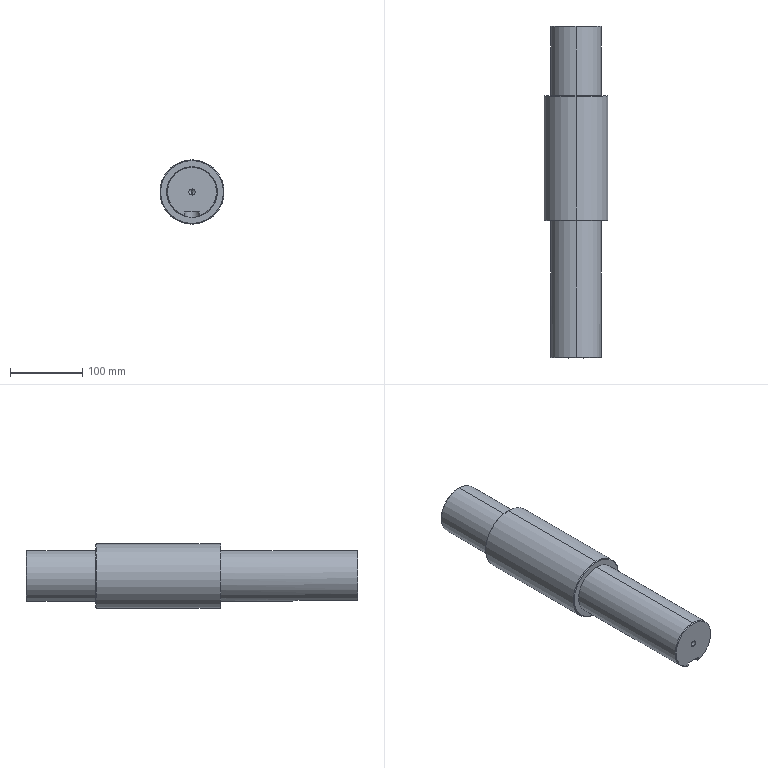Part | SolidWorks | features ICE 3, HoleWzd 2, Chamfer 1, Extrusion 1, MoveFace 1 | 1 solid | 30 faces | box 89 x 459.5 x 89 mm | volume 2162162 mm3 | cone 12 | cylinder 11 | plane 7 | commonest cylinder face diameters 8.5 x4 70 x4 89 x2 20 x1
STEP:
#1=CARTESIAN_POINT('',(0.,405.,-4.25));
#2=VERTEX_POINT('',#1);
#3=CARTESIAN_POINT('',(0.,405.,4.25));
#4=VERTEX_POINT('',#3);
#5=CARTESIAN_POINT('',(0.,405.,0.));
#6=DIRECTION('',(0.,1.,0.));
#7=DIRECTION('',(0.,0.,1.));
#8=AXIS2_PLACEMENT_3D('',#5,#6,#7);
#9=CIRCLE('',#8,4.25);
#10=EDGE_CURVE('',#2,#4,#9,.T.);
#11=ORIENTED_EDGE('',*,*,#10,.F.);
#12=CARTESIAN_POINT('',(0.,425.,-4.25));
#13=VERTEX_POINT('',#12);
#14=CARTESIAN_POINT('',(0.,425.,-4.25));
#15=DIRECTION('',(0.,1.,0.));
#16=VECTOR('',#15,1000.);
#17=LINE('',#14,#16);
#18=EDGE_CURVE('',#2,#13,#17,.T.);
#19=ORIENTED_EDGE('',*,*,#18,.T.);
#20=CARTESIAN_POINT('',(0.,425.,4.25));
#21=VERTEX_POINT('',#20);
#22=CARTESIAN_POINT('',(0.,425.,0.));
#23=DIRECTION('',(0.,1.,0.));
#24=DIRECTION('',(0.,0.,1.));
#25=AXIS2_PLACEMENT_3D('',#22,#23,#24);
#26=CIRCLE('',#25,4.25);
#27=EDGE_CURVE('',#13,#21,#26,.T.);
#28=ORIENTED_EDGE('',*,*,#27,.T.);
#29=CARTESIAN_POINT('',(0.,425.,4.25));
#30=DIRECTION('',(0.,1.,0.));
#31=VECTOR('',#30,1000.);
#32=LINE('',#29,#31);
#33=EDGE_CURVE('',#4,#21,#32,.T.);
#34=ORIENTED_EDGE('',*,*,#33,.F.);
#35=EDGE_LOOP('',(#11,#19,#28,#34));
#36=FACE_OUTER_BOUND('',#35,.T.);
#37=CARTESIAN_POINT('',(0.,425.,0.));
#38=DIRECTION('',(0.,1.,0.));
#39=DIRECTION('',(0.,0.,1.));
#40=AXIS2_PLACEMENT_3D('',#37,#38,#39);
#41=CYLINDRICAL_SURFACE('',#40,4.25);
#42=ADVANCED_FACE('',(#36),#41,.F.);
#43=CARTESIAN_POINT('',(0.,402.446,0.));
#44=VERTEX_POINT('',#43);
#45=CARTESIAN_POINT('',(0.,405.,4.25));
#46=DIRECTION('',(0.,0.515,0.8572));
#47=VECTOR('',#46,1000.);
#48=LINE('',#45,#47);
#49=EDGE_CURVE('',#44,#4,#48,.T.);
#50=ORIENTED_EDGE('',*,*,#49,.F.);
#51=CARTESIAN_POINT('',(0.,405.,-4.25));
#52=DIRECTION('',(0.,0.515,-0.8572));
#53=VECTOR('',#52,1000.);
#54=LINE('',#51,#53);
#55=EDGE_CURVE('',#44,#2,#54,.T.);
#56=ORIENTED_EDGE('',*,*,#55,.T.);
#57=ORIENTED_EDGE('',*,*,#10,.T.);
#58=EDGE_LOOP('',(#50,#56,#57));
#59=FACE_OUTER_BOUND('',#58,.T.);
#60=CARTESIAN_POINT('',(0.,405.,0.));
#61=DIRECTION('',(0.,1.,0.));
#62=DIRECTION('',(0.,0.,1.));
#63=AXIS2_PLACEMENT_3D('',#60,#61,#62);
#64=CONICAL_SURFACE('',#63,4.25,1.03);
#65=ADVANCED_FACE('',(#59),#64,.F.);
#66=CARTESIAN_POINT('',(0.,425.,34.));
#67=VERTEX_POINT('',#66);
#68=CARTESIAN_POINT('',(0.,425.,-34.));
#69=VERTEX_POINT('',#68);
#70=CARTESIAN_POINT('',(0.,425.,0.));
#71=DIRECTION('',(0.,1.,0.));
#72=DIRECTION('',(0.,0.,1.));
#73=AXIS2_PLACEMENT_3D('',#70,#71,#72);
#74=CIRCLE('',#73,34.);
#75=EDGE_CURVE('',#67,#69,#74,.T.);
#76=ORIENTED_EDGE('',*,*,#75,.F.);
#77=CARTESIAN_POINT('',(0.,424.,35.));
#78=VERTEX_POINT('',#77);
#79=CARTESIAN_POINT('',(0.,425.,34.));
#80=DIRECTION('',(0.,-0.7071,0.7071));
#81=VECTOR('',#80,1000.);
#82=LINE('',#79,#81);
#83=EDGE_CURVE('',#67,#78,#82,.T.);
#84=ORIENTED_EDGE('',*,*,#83,.T.);
#85=CARTESIAN_POINT('',(0.,424.,-35.));
#86=VERTEX_POINT('',#85);
#87=CARTESIAN_POINT('',(0.,424.,0.));
#88=DIRECTION('',(0.,-1.,0.));
#89=DIRECTION('',(0.,0.,1.));
#90=AXIS2_PLACEMENT_3D('',#87,#88,#89);
#91=CIRCLE('',#90,35.);
#92=EDGE_CURVE('',#86,#78,#91,.T.);
#93=ORIENTED_EDGE('',*,*,#92,.F.);
#94=CARTESIAN_POINT('',(0.,425.,-34.));
#95=DIRECTION('',(0.,-0.7071,-0.7071));
#96=VECTOR('',#95,1000.);
#97=LINE('',#94,#96);
#98=EDGE_CURVE('',#69,#86,#97,.T.);
#99=ORIENTED_EDGE('',*,*,#98,.F.);
#100=EDGE_LOOP('',(#76,#84,#93,#99));
#101=FACE_OUTER_BOUND('',#100,.T.);
#102=CARTESIAN_POINT('',(0.,425.,0.));
#103=DIRECTION('',(0.,-1.,0.));
#104=DIRECTION('',(0.,0.,-1.));
#105=AXIS2_PLACEMENT_3D('',#102,#103,#104);
#106=CONICAL_SURFACE('',#105,34.,0.7854);
#107=ADVANCED_FACE('',(#101),#106,.T.);
#108=CARTESIAN_POINT('',(0.,328.7,43.5));
#109=VERTEX_POINT('',#108);
#110=CARTESIAN_POINT('',(0.,328.7,-43.5));
#111=VERTEX_POINT('',#110);
#112=CARTESIAN_POINT('',(0.,328.7,0.));
#113=DIRECTION('',(0.,1.,0.));
#114=DIRECTION('',(0.,0.,1.));
#115=AXIS2_PLACEMENT_3D('',#112,#113,#114);
#116=CIRCLE('',#115,43.5);
#117=EDGE_CURVE('',#109,#111,#116,.T.);
#118=ORIENTED_EDGE('',*,*,#117,.F.);
#119=CARTESIAN_POINT('',(0.,327.7,44.5));
#120=VERTEX_POINT('',#119);
#121=CARTESIAN_POINT('',(0.,328.7,43.5));
#122=DIRECTION('',(0.,-0.7071,0.7071));
#123=VECTOR('',#122,1000.);
#124=LINE('',#121,#123);
#125=EDGE_CURVE('',#109,#120,#124,.T.);
#126=ORIENTED_EDGE('',*,*,#125,.T.);
#127=CARTESIAN_POINT('',(0.,327.7,-44.5));
#128=VERTEX_POINT('',#127);
#129=CARTESIAN_POINT('',(0.,327.7,0.));
#130=DIRECTION('',(0.,-1.,0.));
#131=DIRECTION('',(0.,0.,1.));
#132=AXIS2_PLACEMENT_3D('',#129,#130,#131);
#133=CIRCLE('',#132,44.5);
#134=EDGE_CURVE('',#128,#120,#133,.T.);
#135=ORIENTED_EDGE('',*,*,#134,.F.);
#136=CARTESIAN_POINT('',(0.,328.7,-43.5));
#137=DIRECTION('',(0.,-0.7071,-0.7071));
#138=VECTOR('',#137,1000.);
#139=LINE('',#136,#138);
#140=EDGE_CURVE('',#111,#128,#139,.T.);
#141=ORIENTED_EDGE('',*,*,#140,.F.);
#142=EDGE_LOOP('',(#118,#126,#135,#141));
#143=FACE_OUTER_BOUND('',#142,.T.);
#144=CARTESIAN_POINT('',(0.,328.7,0.));
#145=DIRECTION('',(0.,-1.,0.));
#146=DIRECTION('',(0.,0.,-1.));
#147=AXIS2_PLACEMENT_3D('',#144,#145,#146);
#148=CONICAL_SURFACE('',#147,43.5,0.7854);
#149=ADVANCED_FACE('',(#143),#148,.T.);
#150=CARTESIAN_POINT('',(0.,155.3,-43.5));
#151=VERTEX_POINT('',#150);
#152=CARTESIAN_POINT('',(0.,155.3,43.5));
#153=VERTEX_POINT('',#152);
#154=CARTESIAN_POINT('',(0.,155.3,0.));
#155=DIRECTION('',(0.,-1.,0.));
#156=DIRECTION('',(0.,0.,-1.));
#157=AXIS2_PLACEMENT_3D('',#154,#155,#156);
#158=CIRCLE('',#157,43.5);
#159=EDGE_CURVE('',#151,#153,#158,.T.);
#160=ORIENTED_EDGE('',*,*,#159,.F.);
#161=CARTESIAN_POINT('',(0.,156.3,-44.5));
#162=VERTEX_POINT('',#161);
#163=CARTESIAN_POINT('',(0.,155.3,-43.5));
#164=DIRECTION('',(0.,0.7071,-0.7071));
#165=VECTOR('',#164,1000.);
#166=LINE('',#163,#165);
#167=EDGE_CURVE('',#151,#162,#166,.T.);
#168=ORIENTED_EDGE('',*,*,#167,.T.);
#169=CARTESIAN_POINT('',(0.,156.3,44.5));
#170=VERTEX_POINT('',#169);
#171=CARTESIAN_POINT('',(0.,156.3,0.));
#172=DIRECTION('',(0.,1.,0.));
#173=DIRECTION('',(0.,0.,-1.));
#174=AXIS2_PLACEMENT_3D('',#171,#172,#173);
#175=CIRCLE('',#174,44.5);
#176=EDGE_CURVE('',#170,#162,#175,.T.);
#177=ORIENTED_EDGE('',*,*,#176,.F.);
#178=CARTESIAN_POINT('',(0.,155.3,43.5));
#179=DIRECTION('',(0.,0.7071,0.7071));
#180=VECTOR('',#179,1000.);
#181=LINE('',#178,#180);
#182=EDGE_CURVE('',#153,#170,#181,.T.);
#183=ORIENTED_EDGE('',*,*,#182,.F.);
#184=EDGE_LOOP('',(#160,#168,#177,#183));
#185=FACE_OUTER_BOUND('',#184,.T.);
#186=CARTESIAN_POINT('',(0.,155.3,0.));
#187=DIRECTION('',(0.,1.,0.));
#188=DIRECTION('',(0.,0.,1.));
#189=AXIS2_PLACEMENT_3D('',#186,#187,#188);
#190=CONICAL_SURFACE('',#189,43.5,0.7854);
#191=ADVANCED_FACE('',(#185),#190,.T.);
#192=CARTESIAN_POINT('',(0.,-34.5,34.));
#193=VERTEX_POINT('',#192);
#194=CARTESIAN_POINT('',(-10.,-34.5,-32.496));
#195=VERTEX_POINT('',#194);
#196=CARTESIAN_POINT('',(0.,-34.5,0.));
#197=DIRECTION('',(0.,-1.,0.));
#198=DIRECTION('',(0.,0.,1.));
#199=AXIS2_PLACEMENT_3D('',#196,#197,#198);
#200=CIRCLE('',#199,34.);
#201=EDGE_CURVE('',#193,#195,#200,.T.);
#202=ORIENTED_EDGE('',*,*,#201,.F.);
#203=CARTESIAN_POINT('',(0.,-33.5,35.));
#204=VERTEX_POINT('',#203);
#205=CARTESIAN_POINT('',(0.,-34.5,34.));
#206=DIRECTION('',(0.,0.7071,0.7071));
#207=VECTOR('',#206,1000.);
#208=LINE('',#205,#207);
#209=EDGE_CURVE('',#193,#204,#208,.T.);
#210=ORIENTED_EDGE('',*,*,#209,.T.);
#211=CARTESIAN_POINT('',(-10.,-33.5,-33.541));
#212=VERTEX_POINT('',#211);
#213=CARTESIAN_POINT('',(0.,-33.5,0.));
#214=DIRECTION('',(0.,1.,0.));
#215=DIRECTION('',(0.,0.,1.));
#216=AXIS2_PLACEMENT_3D('',#213,#214,#215);
#217=CIRCLE('',#216,35.);
#218=EDGE_CURVE('',#212,#204,#217,.T.);
#219=ORIENTED_EDGE('',*,*,#218,.F.);
#220=CARTESIAN_POINT('',(-10.,-34.5,-32.496));
#221=CARTESIAN_POINT('',(-10.,-34.167,-32.845));
#222=CARTESIAN_POINT('',(-10.,-33.834,-33.193));
#223=CARTESIAN_POINT('',(-10.,-33.5,-33.541));
#224=B_SPLINE_CURVE_WITH_KNOTS('',3,(#220,#221,#222,#223),.UNSPECIFIED.,.F.,.F.,(4,4),(0.,0.001446),.UNSPECIFIED.);
#225=EDGE_CURVE('',#195,#212,#224,.T.);
#226=ORIENTED_EDGE('',*,*,#225,.F.);
#227=EDGE_LOOP('',(#202,#210,#219,#226));
#228=FACE_OUTER_BOUND('',#227,.T.);
#229=CARTESIAN_POINT('',(0.,-34.5,0.));
#230=DIRECTION('',(0.,1.,0.));
#231=DIRECTION('',(0.,0.,1.));
#232=AXIS2_PLACEMENT_3D('',#229,#230,#231);
#233=CONICAL_SURFACE('',#232,34.,0.7854);
#234=ADVANCED_FACE('',(#228),#233,.T.);
#235=CARTESIAN_POINT('',(0.,24.5,4.25));
#236=VERTEX_POINT('',#235);
#237=CARTESIAN_POINT('',(0.,24.5,-4.25));
#238=VERTEX_POINT('',#237);
#239=CARTESIAN_POINT('',(0.,24.5,0.));
#240=DIRECTION('',(0.,-1.,0.));
#241=DIRECTION('',(0.,0.,-1.));
#242=AXIS2_PLACEMENT_3D('',#239,#240,#241);
#243=CIRCLE('',#242,4.25);
#244=EDGE_CURVE('',#236,#238,#243,.T.);
#245=ORIENTED_EDGE('',*,*,#244,.F.);
#246=CARTESIAN_POINT('',(0.,-34.5,4.25));
#247=VERTEX_POINT('',#246);
#248=CARTESIAN_POINT('',(0.,0.,4.25));
#249=DIRECTION('',(0.,-1.,0.));
#250=VECTOR('',#249,1000.);
#251=LINE('',#248,#250);
#252=EDGE_CURVE('',#236,#247,#251,.T.);
#253=ORIENTED_EDGE('',*,*,#252,.T.);
#254=CARTESIAN_POINT('',(0.,-34.5,-4.25));
#255=VERTEX_POINT('',#254);
#256=CARTESIAN_POINT('',(0.,-34.5,0.));
#257=DIRECTION('',(0.,-1.,0.));
#258=DIRECTION('',(0.,0.,-1.));
#259=AXIS2_PLACEMENT_3D('',#256,#257,#258);
#260=CIRCLE('',#259,4.25);
#261=EDGE_CURVE('',#247,#255,#260,.T.);
#262=ORIENTED_EDGE('',*,*,#261,.T.);
#263=CARTESIAN_POINT('',(0.,0.,-4.25));
#264=DIRECTION('',(0.,-1.,0.));
#265=VECTOR('',#264,1000.);
#266=LINE('',#263,#265);
#267=EDGE_CURVE('',#238,#255,#266,.T.);
#268=ORIENTED_EDGE('',*,*,#267,.F.);
#269=EDGE_LOOP('',(#245,#253,#262,#268));
#270=FACE_OUTER_BOUND('',#269,.T.);
#271=CARTESIAN_POINT('',(0.,0.,0.));
#272=DIRECTION('',(0.,-1.,0.));
#273=DIRECTION('',(0.,0.,-1.));
#274=AXIS2_PLACEMENT_3D('',#271,#272,#273);
#275=CYLINDRICAL_SURFACE('',#274,4.25);
#276=ADVANCED_FACE('',(#270),#275,.F.);
#277=CARTESIAN_POINT('',(0.,27.054,0.));
#278=VERTEX_POINT('',#277);
#279=CARTESIAN_POINT('',(0.,24.5,-4.25));
#280=DIRECTION('',(0.,-0.515,-0.8572));
#281=VECTOR('',#280,1000.);
#282=LINE('',#279,#281);
#283=EDGE_CURVE('',#278,#238,#282,.T.);
#284=ORIENTED_EDGE('',*,*,#283,.F.);
#285=CARTESIAN_POINT('',(0.,24.5,4.25));
#286=DIRECTION('',(0.,-0.515,0.8572));
#287=VECTOR('',#286,1000.);
#288=LINE('',#285,#287);
#289=EDGE_CURVE('',#278,#236,#288,.T.);
#290=ORIENTED_EDGE('',*,*,#289,.T.);
#291=ORIENTED_EDGE('',*,*,#244,.T.);
#292=EDGE_LOOP('',(#284,#290,#291));
#293=FACE_OUTER_BOUND('',#292,.T.);
#294=CARTESIAN_POINT('',(0.,24.5,0.));
#295=DIRECTION('',(0.,-1.,0.));
#296=DIRECTION('',(0.,0.,-1.));
#297=AXIS2_PLACEMENT_3D('',#294,#295,#296);
#298=CONICAL_SURFACE('',#297,4.25,1.03);
#299=ADVANCED_FACE('',(#293),#298,.F.);
#300=CARTESIAN_POINT('',(0.,155.3,-35.));
#301=VERTEX_POINT('',#300);
#302=CARTESIAN_POINT('',(0.,155.3,35.));
#303=VERTEX_POINT('',#302);
#304=CARTESIAN_POINT('',(0.,155.3,0.));
#305=DIRECTION('',(0.,-1.,0.));
#306=DIRECTION('',(0.,0.,-1.));
#307=AXIS2_PLACEMENT_3D('',#304,#305,#306);
#308=CIRCLE('',#307,35.);
#309=EDGE_CURVE('',#301,#303,#308,.T.);
#310=ORIENTED_EDGE('',*,*,#309,.T.);
#311=CARTESIAN_POINT('',(0.,155.3,35.));
#312=DIRECTION('',(0.,-1.,0.));
#313=VECTOR('',#312,1000.);
#314=LINE('',#311,#313);
#315=EDGE_CURVE('',#303,#204,#314,.T.);
#316=ORIENTED_EDGE('',*,*,#315,.T.);
#317=CARTESIAN_POINT('',(10.,-33.5,-33.541));
#318=VERTEX_POINT('',#317);
#319=CARTESIAN_POINT('',(0.,-33.5,0.));
#320=DIRECTION('',(0.,1.,0.));
#321=DIRECTION('',(0.,0.,1.));
#322=AXIS2_PLACEMENT_3D('',#319,#320,#321);
#323=CIRCLE('',#322,35.);
#324=EDGE_CURVE('',#204,#318,#323,.T.);
#325=ORIENTED_EDGE('',*,*,#324,.T.);
#326=CARTESIAN_POINT('',(10.,47.,-33.541));
#327=VERTEX_POINT('',#326);
#328=CARTESIAN_POINT('',(10.,155.3,-33.541));
#329=DIRECTION('',(0.,-1.,0.));
#330=VECTOR('',#329,1000.);
#331=LINE('',#328,#330);
#332=EDGE_CURVE('',#327,#318,#331,.T.);
#333=ORIENTED_EDGE('',*,*,#332,.F.);
#334=CARTESIAN_POINT('',(0.,57.,-35.));
#335=VERTEX_POINT('',#334);
#336=CARTESIAN_POINT('',(0.,57.,-35.));
#337=CARTESIAN_POINT('',(0.6556,57.,-35.));
#338=CARTESIAN_POINT('',(1.322,56.934,-34.981));
#339=CARTESIAN_POINT('',(2.606,56.677,-34.909));
#340=CARTESIAN_POINT('',(3.23,56.487,-34.856));
#341=CARTESIAN_POINT('',(4.141,56.108,-34.756));
#342=CARTESIAN_POINT('',(4.439,55.966,-34.719));
#343=CARTESIAN_POINT('',(5.015,55.658,-34.64));
#344=CARTESIAN_POINT('',(5.293,55.49,-34.598));
#345=CARTESIAN_POINT('',(5.833,55.129,-34.512));
#346=CARTESIAN_POINT('',(6.093,54.936,-34.466));
#347=CARTESIAN_POINT('',(6.597,54.522,-34.374));
#348=CARTESIAN_POINT('',(6.841,54.301,-34.326));
#349=CARTESIAN_POINT('',(7.534,53.608,-34.183));
#350=CARTESIAN_POINT('',(7.945,53.108,-34.088));
#351=CARTESIAN_POINT('',(8.668,52.029,-33.912));
#352=CARTESIAN_POINT('',(8.982,51.444,-33.829));
#353=CARTESIAN_POINT('',(9.483,50.24,-33.692));
#354=CARTESIAN_POINT('',(9.674,49.617,-33.637));
#355=CARTESIAN_POINT('',(9.868,48.65,-33.58));
#356=CARTESIAN_POINT('',(9.918,48.321,-33.565));
#357=CARTESIAN_POINT('',(9.984,47.663,-33.546));
#358=CARTESIAN_POINT('',(10.,47.332,-33.541));
#359=CARTESIAN_POINT('',(10.,47.,-33.541));
#360=B_SPLINE_CURVE_WITH_KNOTS('',3,(#336,#337,#338,#339,#340,#341,#342,#343,#344,#345,#346,#347,#348,#349,#350,#351,#352,#353,#354,#355,#356,#357,#358,#359),.UNSPECIFIED.,.F.,.F.,(4,2,2,2,2,2,2,2,2,2,2,4),(0.01572,0.01768,0.01964,0.02062,0.02161,0.02259,0.02357,0.02553,0.02749,0.02946,0.03044,0.03142),.UNSPECIFIED.);
#361=EDGE_CURVE('',#335,#327,#360,.T.);
#362=ORIENTED_EDGE('',*,*,#361,.F.);
#363=CARTESIAN_POINT('',(0.,155.3,-35.));
#364=DIRECTION('',(0.,-1.,0.));
#365=VECTOR('',#364,1000.);
#366=LINE('',#363,#365);
#367=EDGE_CURVE('',#301,#335,#366,.T.);
#368=ORIENTED_EDGE('',*,*,#367,.F.);
#369=EDGE_LOOP('',(#310,#316,#325,#333,#362,#368));
#370=FACE_OUTER_BOUND('',#369,.T.);
#371=CARTESIAN_POINT('',(0.,155.3,0.));
#372=DIRECTION('',(0.,-1.,0.));
#373=DIRECTION('',(0.,0.,-1.));
#374=AXIS2_PLACEMENT_3D('',#371,#372,#373);
#375=CYLINDRICAL_SURFACE('',#374,35.);
#376=ADVANCED_FACE('',(#370),#375,.T.);
#377=CARTESIAN_POINT('',(0.,328.7,35.));
#378=VERTEX_POINT('',#377);
#379=CARTESIAN_POINT('',(0.,328.7,-35.));
#380=VERTEX_POINT('',#379);
#381=CARTESIAN_POINT('',(0.,328.7,0.));
#382=DIRECTION('',(0.,1.,0.));
#383=DIRECTION('',(0.,0.,1.));
#384=AXIS2_PLACEMENT_3D('',#381,#382,#383);
#385=CIRCLE('',#384,35.);
#386=EDGE_CURVE('',#378,#380,#385,.T.);
#387=ORIENTED_EDGE('',*,*,#386,.T.);
#388=CARTESIAN_POINT('',(0.,328.7,-35.));
#389=DIRECTION('',(0.,1.,0.));
#390=VECTOR('',#389,1000.);
#391=LINE('',#388,#390);
#392=EDGE_CURVE('',#380,#86,#391,.T.);
#393=ORIENTED_EDGE('',*,*,#392,.T.);
#394=ORIENTED_EDGE('',*,*,#92,.T.);
#395=CARTESIAN_POINT('',(0.,328.7,35.));
#396=DIRECTION('',(0.,1.,0.));
#397=VECTOR('',#396,1000.);
#398=LINE('',#395,#397);
#399=EDGE_CURVE('',#378,#78,#398,.T.);
#400=ORIENTED_EDGE('',*,*,#399,.F.);
#401=EDGE_LOOP('',(#387,#393,#394,#400));
#402=FACE_OUTER_BOUND('',#401,.T.);
#403=CARTESIAN_POINT('',(0.,328.7,0.));
#404=DIRECTION('',(0.,1.,0.));
#405=DIRECTION('',(0.,0.,1.));
#406=AXIS2_PLACEMENT_3D('',#403,#404,#405);
#407=CYLINDRICAL_SURFACE('',#406,35.);
#408=ADVANCED_FACE('',(#402),#407,.T.);
#409=ORIENTED_EDGE('',*,*,#134,.T.);
#410=CARTESIAN_POINT('',(0.,425.,44.5));
#411=DIRECTION('',(0.,-1.,0.));
#412=VECTOR('',#411,1000.);
#413=LINE('',#410,#412);
#414=EDGE_CURVE('',#120,#170,#413,.T.);
#415=ORIENTED_EDGE('',*,*,#414,.T.);
#416=ORIENTED_EDGE('',*,*,#176,.T.);
#417=CARTESIAN_POINT('',(0.,425.,-44.5));
#418=DIRECTION('',(0.,-1.,0.));
#419=VECTOR('',#418,1000.);
#420=LINE('',#417,#419);
#421=EDGE_CURVE('',#128,#162,#420,.T.);
#422=ORIENTED_EDGE('',*,*,#421,.F.);
#423=EDGE_LOOP('',(#409,#415,#416,#422));
#424=FACE_OUTER_BOUND('',#423,.T.);
#425=CARTESIAN_POINT('',(0.,425.,0.));
#426=DIRECTION('',(0.,-1.,0.));
#427=DIRECTION('',(0.,0.,-1.));
#428=AXIS2_PLACEMENT_3D('',#425,#426,#427);
#429=CYLINDRICAL_SURFACE('',#428,44.5);
#430=ADVANCED_FACE('',(#424),#429,.T.);
#431=ORIENTED_EDGE('',*,*,#414,.F.);
#432=CARTESIAN_POINT('',(0.,327.7,0.));
#433=DIRECTION('',(0.,-1.,0.));
#434=DIRECTION('',(0.,0.,1.));
#435=AXIS2_PLACEMENT_3D('',#432,#433,#434);
#436=CIRCLE('',#435,44.5);
#437=EDGE_CURVE('',#120,#128,#436,.T.);
#438=ORIENTED_EDGE('',*,*,#437,.T.);
#439=ORIENTED_EDGE('',*,*,#421,.T.);
#440=CARTESIAN_POINT('',(0.,156.3,0.));
#441=DIRECTION('',(0.,1.,0.));
#442=DIRECTION('',(0.,0.,-1.));
#443=AXIS2_PLACEMENT_3D('',#440,#441,#442);
#444=CIRCLE('',#443,44.5);
#445=EDGE_CURVE('',#162,#170,#444,.T.);
#446=ORIENTED_EDGE('',*,*,#445,.T.);
#447=EDGE_LOOP('',(#431,#438,#439,#446));
#448=FACE_OUTER_BOUND('',#447,.T.);
#449=CARTESIAN_POINT('',(0.,425.,0.));
#450=DIRECTION('',(0.,-1.,0.));
#451=DIRECTION('',(0.,0.,-1.));
#452=AXIS2_PLACEMENT_3D('',#449,#450,#451);
#453=CYLINDRICAL_SURFACE('',#452,44.5);
#454=ADVANCED_FACE('',(#448),#453,.T.);
#455=CARTESIAN_POINT('',(0.,328.7,0.));
#456=DIRECTION('',(0.,1.,0.));
#457=DIRECTION('',(0.,0.,1.));
#458=AXIS2_PLACEMENT_3D('',#455,#456,#457);
#459=CIRCLE('',#458,43.5);
#460=EDGE_CURVE('',#111,#109,#459,.T.);
#461=ORIENTED_EDGE('',*,*,#460,.T.);
#462=ORIENTED_EDGE('',*,*,#117,.T.);
#463=EDGE_LOOP('',(#461,#462));
#464=FACE_OUTER_BOUND('',#463,.T.);
#465=ORIENTED_EDGE('',*,*,#386,.F.);
#466=CARTESIAN_POINT('',(0.,328.7,0.));
#467=DIRECTION('',(0.,1.,0.));
#468=DIRECTION('',(0.,0.,1.));
#469=AXIS2_PLACEMENT_3D('',#466,#467,#468);
#470=CIRCLE('',#469,35.);
#471=EDGE_CURVE('',#380,#378,#470,.T.);
#472=ORIENTED_EDGE('',*,*,#471,.F.);
#473=EDGE_LOOP('',(#465,#472));
#474=FACE_BOUND('',#473,.T.);
#475=CARTESIAN_POINT('',(0.,328.7,0.));
#476=DIRECTION('',(0.,1.,0.));
#477=DIRECTION('',(0.,0.,1.));
#478=AXIS2_PLACEMENT_3D('',#475,#476,#477);
#479=PLANE('',#478);
#480=ADVANCED_FACE('',(#464,#474),#479,.T.);
#481=ORIENTED_EDGE('',*,*,#392,.F.);
#482=ORIENTED_EDGE('',*,*,#471,.T.);
#483=ORIENTED_EDGE('',*,*,#399,.T.);
#484=CARTESIAN_POINT('',(0.,424.,0.));
#485=DIRECTION('',(0.,-1.,0.));
#486=DIRECTION('',(0.,0.,1.));
#487=AXIS2_PLACEMENT_3D('',#484,#485,#486);
#488=CIRCLE('',#487,35.);
#489=EDGE_CURVE('',#78,#86,#488,.T.);
#490=ORIENTED_EDGE('',*,*,#489,.T.);
#491=EDGE_LOOP('',(#481,#482,#483,#490));
#492=FACE_OUTER_BOUND('',#491,.T.);
#493=CARTESIAN_POINT('',(0.,328.7,0.));
#494=DIRECTION('',(0.,1.,0.));
#495=DIRECTION('',(0.,0.,1.));
#496=AXIS2_PLACEMENT_3D('',#493,#494,#495);
#497=CYLINDRICAL_SURFACE('',#496,35.);
#498=ADVANCED_FACE('',(#492),#497,.T.);
#499=CARTESIAN_POINT('',(0.,425.,0.));
#500=DIRECTION('',(0.,1.,0.));
#501=DIRECTION('',(0.,0.,1.));
#502=AXIS2_PLACEMENT_3D('',#499,#500,#501);
#503=CIRCLE('',#502,4.25);
#504=EDGE_CURVE('',#21,#13,#503,.T.);
#505=ORIENTED_EDGE('',*,*,#504,.F.);
#506=ORIENTED_EDGE('',*,*,#27,.F.);
#507=EDGE_LOOP('',(#505,#506));
#508=FACE_BOUND('',#507,.T.);
#509=CARTESIAN_POINT('',(0.,425.,0.));
#510=DIRECTION('',(0.,1.,0.));
#511=DIRECTION('',(0.,0.,1.));
#512=AXIS2_PLACEMENT_3D('',#509,#510,#511);
#513=CIRCLE('',#512,34.);
#514=EDGE_CURVE('',#69,#67,#513,.T.);
#515=ORIENTED_EDGE('',*,*,#514,.T.);
#516=ORIENTED_EDGE('',*,*,#75,.T.);
#517=EDGE_LOOP('',(#515,#516));
#518=FACE_OUTER_BOUND('',#517,.T.);
#519=CARTESIAN_POINT('',(0.,425.,0.));
#520=DIRECTION('',(0.,1.,0.));
#521=DIRECTION('',(0.,0.,1.));
#522=AXIS2_PLACEMENT_3D('',#519,#520,#521);
#523=PLANE('',#522);
#524=ADVANCED_FACE('',(#508,#518),#523,.T.);
#525=CARTESIAN_POINT('',(0.,155.3,0.));
#526=DIRECTION('',(0.,-1.,0.));
#527=DIRECTION('',(0.,0.,-1.));
#528=AXIS2_PLACEMENT_3D('',#525,#526,#527);
#529=CIRCLE('',#528,43.5);
#530=EDGE_CURVE('',#153,#151,#529,.T.);
#531=ORIENTED_EDGE('',*,*,#530,.T.);
#532=ORIENTED_EDGE('',*,*,#159,.T.);
#533=EDGE_LOOP('',(#531,#532));
#534=FACE_OUTER_BOUND('',#533,.T.);
#535=ORIENTED_EDGE('',*,*,#309,.F.);
#536=CARTESIAN_POINT('',(0.,155.3,0.));
#537=DIRECTION('',(0.,-1.,0.));
#538=DIRECTION('',(0.,0.,-1.));
#539=AXIS2_PLACEMENT_3D('',#536,#537,#538);
#540=CIRCLE('',#539,35.);
#541=EDGE_CURVE('',#303,#301,#540,.T.);
#542=ORIENTED_EDGE('',*,*,#541,.F.);
#543=EDGE_LOOP('',(#535,#542));
#544=FACE_BOUND('',#543,.T.);
#545=CARTESIAN_POINT('',(0.,155.3,0.));
#546=DIRECTION('',(0.,-1.,0.));
#547=DIRECTION('',(0.,0.,-1.));
#548=AXIS2_PLACEMENT_3D('',#545,#546,#547);
#549=PLANE('',#548);
#550=ADVANCED_FACE('',(#534,#544),#549,.T.);
#551=ORIENTED_EDGE('',*,*,#315,.F.);
#552=ORIENTED_EDGE('',*,*,#541,.T.);
#553=ORIENTED_EDGE('',*,*,#367,.T.);
#554=CARTESIAN_POINT('',(-10.,47.,-33.541));
#555=VERTEX_POINT('',#554);
#556=CARTESIAN_POINT('',(-10.,47.,-33.541));
#557=CARTESIAN_POINT('',(-10.,47.665,-33.541));
#558=CARTESIAN_POINT('',(-9.934,48.317,-33.561));
#559=CARTESIAN_POINT('',(-9.742,49.28,-33.617));
#560=CARTESIAN_POINT('',(-9.662,49.598,-33.64));
#561=CARTESIAN_POINT('',(-9.47,50.228,-33.695));
#562=CARTESIAN_POINT('',(-9.358,50.54,-33.726));
#563=CARTESIAN_POINT('',(-8.981,51.447,-33.829));
#564=CARTESIAN_POINT('',(-8.673,52.02,-33.91));
#565=CARTESIAN_POINT('',(-8.129,52.834,-34.044));
#566=CARTESIAN_POINT('',(-7.932,53.099,-34.09));
#567=CARTESIAN_POINT('',(-7.516,53.604,-34.184));
#568=CARTESIAN_POINT('',(-7.298,53.845,-34.232));
#569=CARTESIAN_POINT('',(-6.609,54.533,-34.374));
#570=CARTESIAN_POINT('',(-6.108,54.945,-34.467));
#571=CARTESIAN_POINT('',(-5.015,55.677,-34.643));
#572=CARTESIAN_POINT('',(-4.438,55.985,-34.723));
#573=CARTESIAN_POINT('',(-3.536,56.36,-34.822));
#574=CARTESIAN_POINT('',(-3.229,56.47,-34.852));
#575=CARTESIAN_POINT('',(-2.6,56.662,-34.905));
#576=CARTESIAN_POINT('',(-2.278,56.743,-34.927));
#577=CARTESIAN_POINT('',(-1.308,56.936,-34.982));
#578=CARTESIAN_POINT('',(-0.6564,57.,-35.));
#579=CARTESIAN_POINT('',(0.,57.,-35.));
#580=B_SPLINE_CURVE_WITH_KNOTS('',3,(#556,#557,#558,#559,#560,#561,#562,#563,#564,#565,#566,#567,#568,#569,#570,#571,#572,#573,#574,#575,#576,#577,#578,#579),.UNSPECIFIED.,.F.,.F.,(4,2,2,2,2,2,2,2,2,2,2,4),(0.,0.001965,0.002947,0.00393,0.005894,0.006877,0.007859,0.009824,0.01179,0.01277,0.01375,0.01572),.UNSPECIFIED.);
#581=EDGE_CURVE('',#555,#335,#580,.T.);
#582=ORIENTED_EDGE('',*,*,#581,.F.);
#583=CARTESIAN_POINT('',(-10.,155.3,-33.541));
#584=DIRECTION('',(0.,1.,0.));
#585=VECTOR('',#584,1000.);
#586=LINE('',#583,#585);
#587=EDGE_CURVE('',#212,#555,#586,.T.);
#588=ORIENTED_EDGE('',*,*,#587,.F.);
#589=ORIENTED_EDGE('',*,*,#218,.T.);
#590=EDGE_LOOP('',(#551,#552,#553,#582,#588,#589));
#591=FACE_OUTER_BOUND('',#590,.T.);
#592=CARTESIAN_POINT('',(0.,155.3,0.));
#593=DIRECTION('',(0.,-1.,0.));
#594=DIRECTION('',(0.,0.,-1.));
#595=AXIS2_PLACEMENT_3D('',#592,#593,#594);
#596=CYLINDRICAL_SURFACE('',#595,35.);
#597=ADVANCED_FACE('',(#591),#596,.T.);
#598=CARTESIAN_POINT('',(0.,-34.5,0.));
#599=DIRECTION('',(0.,-1.,0.));
#600=DIRECTION('',(0.,0.,-1.));
#601=AXIS2_PLACEMENT_3D('',#598,#599,#600);
#602=CIRCLE('',#601,4.25);
#603=EDGE_CURVE('',#255,#247,#602,.T.);
#604=ORIENTED_EDGE('',*,*,#603,.F.);
#605=ORIENTED_EDGE('',*,*,#261,.F.);
#606=EDGE_LOOP('',(#604,#605));
#607=FACE_BOUND('',#606,.T.);
#608=CARTESIAN_POINT('',(10.,-34.5,-27.5));
#609=VERTEX_POINT('',#608);
#610=CARTESIAN_POINT('',(10.,-34.5,-32.496));
#611=VERTEX_POINT('',#610);
#612=CARTESIAN_POINT('',(10.,-34.5,-27.5));
#613=DIRECTION('',(0.,0.,-1.));
#614=VECTOR('',#613,1000.);
#615=LINE('',#612,#614);
#616=EDGE_CURVE('',#609,#611,#615,.T.);
#617=ORIENTED_EDGE('',*,*,#616,.T.);
#618=CARTESIAN_POINT('',(0.,-34.5,0.));
#619=DIRECTION('',(0.,-1.,0.));
#620=DIRECTION('',(0.,0.,1.));
#621=AXIS2_PLACEMENT_3D('',#618,#619,#620);
#622=CIRCLE('',#621,34.);
#623=EDGE_CURVE('',#611,#193,#622,.T.);
#624=ORIENTED_EDGE('',*,*,#623,.T.);
#625=ORIENTED_EDGE('',*,*,#201,.T.);
#626=CARTESIAN_POINT('',(-10.,-34.5,-27.5));
#627=VERTEX_POINT('',#626);
#628=CARTESIAN_POINT('',(-10.,-34.5,-27.5));
#629=DIRECTION('',(0.,0.,-1.));
#630=VECTOR('',#629,1000.);
#631=LINE('',#628,#630);
#632=EDGE_CURVE('',#627,#195,#631,.T.);
#633=ORIENTED_EDGE('',*,*,#632,.F.);
#634=CARTESIAN_POINT('',(0.,-34.5,-27.5));
#635=DIRECTION('',(-1.,0.,0.));
#636=VECTOR('',#635,1000.);
#637=LINE('',#634,#636);
#638=EDGE_CURVE('',#609,#627,#637,.T.);
#639=ORIENTED_EDGE('',*,*,#638,.F.);
#640=EDGE_LOOP('',(#617,#624,#625,#633,#639));
#641=FACE_OUTER_BOUND('',#640,.T.);
#642=CARTESIAN_POINT('',(0.,-34.5,0.));
#643=DIRECTION('',(0.,1.,0.));
#644=DIRECTION('',(0.,0.,1.));
#645=AXIS2_PLACEMENT_3D('',#642,#643,#644);
#646=PLANE('',#645);
#647=ADVANCED_FACE('',(#607,#641),#646,.F.);
#648=ORIENTED_EDGE('',*,*,#638,.T.);
#649=CARTESIAN_POINT('',(-10.,47.,-27.5));
#650=VERTEX_POINT('',#649);
#651=CARTESIAN_POINT('',(-10.,0.,-27.5));
#652=DIRECTION('',(0.,1.,0.));
#653=VECTOR('',#652,1000.);
#654=LINE('',#651,#653);
#655=EDGE_CURVE('',#627,#650,#654,.T.);
#656=ORIENTED_EDGE('',*,*,#655,.T.);
#657=CARTESIAN_POINT('',(10.,47.,-27.5));
#658=VERTEX_POINT('',#657);
#659=CARTESIAN_POINT('',(0.,47.,-27.5));
#660=DIRECTION('',(0.,0.,-1.));
#661=DIRECTION('',(-1.,0.,0.));
#662=AXIS2_PLACEMENT_3D('',#659,#660,#661);
#663=CIRCLE('',#662,10.);
#664=EDGE_CURVE('',#650,#658,#663,.T.);
#665=ORIENTED_EDGE('',*,*,#664,.T.);
#666=CARTESIAN_POINT('',(10.,0.,-27.5));
#667=DIRECTION('',(0.,-1.,0.));
#668=VECTOR('',#667,1000.);
#669=LINE('',#666,#668);
#670=EDGE_CURVE('',#658,#609,#669,.T.);
#671=ORIENTED_EDGE('',*,*,#670,.T.);
#672=EDGE_LOOP('',(#648,#656,#665,#671));
#673=FACE_OUTER_BOUND('',#672,.T.);
#674=CARTESIAN_POINT('',(0.,0.,-27.5));
#675=DIRECTION('',(0.,0.,-1.));
#676=DIRECTION('',(-1.,0.,0.));
#677=AXIS2_PLACEMENT_3D('',#674,#675,#676);
#678=PLANE('',#677);
#679=ADVANCED_FACE('',(#673),#678,.T.);
#680=ORIENTED_EDGE('',*,*,#332,.T.);
#681=CARTESIAN_POINT('',(10.,-33.5,-33.541));
#682=CARTESIAN_POINT('',(10.,-33.834,-33.193));
#683=CARTESIAN_POINT('',(10.,-34.167,-32.845));
#684=CARTESIAN_POINT('',(10.,-34.5,-32.496));
#685=B_SPLINE_CURVE_WITH_KNOTS('',3,(#681,#682,#683,#684),.UNSPECIFIED.,.F.,.F.,(4,4),(0.,0.001446),.UNSPECIFIED.);
#686=EDGE_CURVE('',#318,#611,#685,.T.);
#687=ORIENTED_EDGE('',*,*,#686,.T.);
#688=ORIENTED_EDGE('',*,*,#616,.F.);
#689=ORIENTED_EDGE('',*,*,#670,.F.);
#690=CARTESIAN_POINT('',(10.,47.,-27.5));
#691=DIRECTION('',(0.,0.,-1.));
#692=VECTOR('',#691,1000.);
#693=LINE('',#690,#692);
#694=EDGE_CURVE('',#658,#327,#693,.T.);
#695=ORIENTED_EDGE('',*,*,#694,.T.);
#696=EDGE_LOOP('',(#680,#687,#688,#689,#695));
#697=FACE_OUTER_BOUND('',#696,.T.);
#698=CARTESIAN_POINT('',(10.,0.,-27.5));
#699=DIRECTION('',(1.,0.,0.));
#700=DIRECTION('',(0.,0.,-1.));
#701=AXIS2_PLACEMENT_3D('',#698,#699,#700);
#702=PLANE('',#701);
#703=ADVANCED_FACE('',(#697),#702,.F.);
#704=CARTESIAN_POINT('',(-10.,47.,-27.5));
#705=DIRECTION('',(0.,0.,-1.));
#706=VECTOR('',#705,1000.);
#707=LINE('',#704,#706);
#708=EDGE_CURVE('',#650,#555,#707,.T.);
#709=ORIENTED_EDGE('',*,*,#708,.T.);
#710=ORIENTED_EDGE('',*,*,#581,.T.);
#711=ORIENTED_EDGE('',*,*,#361,.T.);
#712=ORIENTED_EDGE('',*,*,#694,.F.);
#713=ORIENTED_EDGE('',*,*,#664,.F.);
#714=EDGE_LOOP('',(#709,#710,#711,#712,#713));
#715=FACE_OUTER_BOUND('',#714,.T.);
#716=CARTESIAN_POINT('',(0.,47.,-27.5));
#717=DIRECTION('',(0.,0.,-1.));
#718=DIRECTION('',(-1.,0.,0.));
#719=AXIS2_PLACEMENT_3D('',#716,#717,#718);
#720=CYLINDRICAL_SURFACE('',#719,10.);
#721=ADVANCED_FACE('',(#715),#720,.F.);
#722=ORIENTED_EDGE('',*,*,#632,.T.);
#723=ORIENTED_EDGE('',*,*,#225,.T.);
#724=ORIENTED_EDGE('',*,*,#587,.T.);
#725=ORIENTED_EDGE('',*,*,#708,.F.);
#726=ORIENTED_EDGE('',*,*,#655,.F.);
#727=EDGE_LOOP('',(#722,#723,#724,#725,#726));
#728=FACE_OUTER_BOUND('',#727,.T.);
#729=CARTESIAN_POINT('',(-10.,0.,-27.5));
#730=DIRECTION('',(-1.,0.,0.));
#731=DIRECTION('',(0.,0.,1.));
#732=AXIS2_PLACEMENT_3D('',#729,#730,#731);
#733=PLANE('',#732);
#734=ADVANCED_FACE('',(#728),#733,.F.);
#735=ORIENTED_EDGE('',*,*,#289,.F.);
#736=ORIENTED_EDGE('',*,*,#283,.T.);
#737=CARTESIAN_POINT('',(0.,24.5,0.));
#738=DIRECTION('',(0.,-1.,0.));
#739=DIRECTION('',(0.,0.,-1.));
#740=AXIS2_PLACEMENT_3D('',#737,#738,#739);
#741=CIRCLE('',#740,4.25);
#742=EDGE_CURVE('',#238,#236,#741,.T.);
#743=ORIENTED_EDGE('',*,*,#742,.T.);
#744=EDGE_LOOP('',(#735,#736,#743));
#745=FACE_OUTER_BOUND('',#744,.T.);
#746=CARTESIAN_POINT('',(0.,24.5,0.));
#747=DIRECTION('',(0.,-1.,0.));
#748=DIRECTION('',(0.,0.,-1.));
#749=AXIS2_PLACEMENT_3D('',#746,#747,#748);
#750=CONICAL_SURFACE('',#749,4.25,1.03);
#751=ADVANCED_FACE('',(#745),#750,.F.);
#752=ORIENTED_EDGE('',*,*,#252,.F.);
#753=ORIENTED_EDGE('',*,*,#742,.F.);
#754=ORIENTED_EDGE('',*,*,#267,.T.);
#755=ORIENTED_EDGE('',*,*,#603,.T.);
#756=EDGE_LOOP('',(#752,#753,#754,#755));
#757=FACE_OUTER_BOUND('',#756,.T.);
#758=CARTESIAN_POINT('',(0.,0.,0.));
#759=DIRECTION('',(0.,-1.,0.));
#760=DIRECTION('',(0.,0.,-1.));
#761=AXIS2_PLACEMENT_3D('',#758,#759,#760);
#762=CYLINDRICAL_SURFACE('',#761,4.25);
#763=ADVANCED_FACE('',(#757),#762,.F.);
#764=ORIENTED_EDGE('',*,*,#209,.F.);
#765=ORIENTED_EDGE('',*,*,#623,.F.);
#766=ORIENTED_EDGE('',*,*,#686,.F.);
#767=ORIENTED_EDGE('',*,*,#324,.F.);
#768=EDGE_LOOP('',(#764,#765,#766,#767));
#769=FACE_OUTER_BOUND('',#768,.T.);
#770=CARTESIAN_POINT('',(0.,-34.5,0.));
#771=DIRECTION('',(0.,1.,0.));
#772=DIRECTION('',(0.,0.,1.));
#773=AXIS2_PLACEMENT_3D('',#770,#771,#772);
#774=CONICAL_SURFACE('',#773,34.,0.7854);
#775=ADVANCED_FACE('',(#769),#774,.T.);
#776=ORIENTED_EDGE('',*,*,#167,.F.);
#777=ORIENTED_EDGE('',*,*,#530,.F.);
#778=ORIENTED_EDGE('',*,*,#182,.T.);
#779=ORIENTED_EDGE('',*,*,#445,.F.);
#780=EDGE_LOOP('',(#776,#777,#778,#779));
#781=FACE_OUTER_BOUND('',#780,.T.);
#782=CARTESIAN_POINT('',(0.,155.3,0.));
#783=DIRECTION('',(0.,1.,0.));
#784=DIRECTION('',(0.,0.,1.));
#785=AXIS2_PLACEMENT_3D('',#782,#783,#784);
#786=CONICAL_SURFACE('',#785,43.5,0.7854);
#787=ADVANCED_FACE('',(#781),#786,.T.);
#788=ORIENTED_EDGE('',*,*,#125,.F.);
#789=ORIENTED_EDGE('',*,*,#460,.F.);
#790=ORIENTED_EDGE('',*,*,#140,.T.);
#791=ORIENTED_EDGE('',*,*,#437,.F.);
#792=EDGE_LOOP('',(#788,#789,#790,#791));
#793=FACE_OUTER_BOUND('',#792,.T.);
#794=CARTESIAN_POINT('',(0.,328.7,0.));
#795=DIRECTION('',(0.,-1.,0.));
#796=DIRECTION('',(0.,0.,-1.));
#797=AXIS2_PLACEMENT_3D('',#794,#795,#796);
#798=CONICAL_SURFACE('',#797,43.5,0.7854);
#799=ADVANCED_FACE('',(#793),#798,.T.);
#800=ORIENTED_EDGE('',*,*,#83,.F.);
#801=ORIENTED_EDGE('',*,*,#514,.F.);
#802=ORIENTED_EDGE('',*,*,#98,.T.);
#803=ORIENTED_EDGE('',*,*,#489,.F.);
#804=EDGE_LOOP('',(#800,#801,#802,#803));
#805=FACE_OUTER_BOUND('',#804,.T.);
#806=CARTESIAN_POINT('',(0.,425.,0.));
#807=DIRECTION('',(0.,-1.,0.));
#808=DIRECTION('',(0.,0.,-1.));
#809=AXIS2_PLACEMENT_3D('',#806,#807,#808);
#810=CONICAL_SURFACE('',#809,34.,0.7854);
#811=ADVANCED_FACE('',(#805),#810,.T.);
#812=ORIENTED_EDGE('',*,*,#55,.F.);
#813=ORIENTED_EDGE('',*,*,#49,.T.);
#814=CARTESIAN_POINT('',(0.,405.,0.));
#815=DIRECTION('',(0.,1.,0.));
#816=DIRECTION('',(0.,0.,1.));
#817=AXIS2_PLACEMENT_3D('',#814,#815,#816);
#818=CIRCLE('',#817,4.25);
#819=EDGE_CURVE('',#4,#2,#818,.T.);
#820=ORIENTED_EDGE('',*,*,#819,.T.);
#821=EDGE_LOOP('',(#812,#813,#820));
#822=FACE_OUTER_BOUND('',#821,.T.);
#823=CARTESIAN_POINT('',(0.,405.,0.));
#824=DIRECTION('',(0.,1.,0.));
#825=DIRECTION('',(0.,0.,1.));
#826=AXIS2_PLACEMENT_3D('',#823,#824,#825);
#827=CONICAL_SURFACE('',#826,4.25,1.03);
#828=ADVANCED_FACE('',(#822),#827,.F.);
#829=ORIENTED_EDGE('',*,*,#18,.F.);
#830=ORIENTED_EDGE('',*,*,#819,.F.);
#831=ORIENTED_EDGE('',*,*,#33,.T.);
#832=ORIENTED_EDGE('',*,*,#504,.T.);
#833=EDGE_LOOP('',(#829,#830,#831,#832));
#834=FACE_OUTER_BOUND('',#833,.T.);
#835=CARTESIAN_POINT('',(0.,425.,0.));
#836=DIRECTION('',(0.,1.,0.));
#837=DIRECTION('',(0.,0.,1.));
#838=AXIS2_PLACEMENT_3D('',#835,#836,#837);
#839=CYLINDRICAL_SURFACE('',#838,4.25);
#840=ADVANCED_FACE('',(#834),#839,.F.);
#841=CLOSED_SHELL('',(#42,#65,#107,#149,#191,#234,#276,#299,#376,#408,#430,#454,#480,#498,#524,#550,#597,#647,#679,#703,#721,#734,#751,#763,#775,#787,#799,#811,#828,#840));
#842=MANIFOLD_SOLID_BREP('',#841);
#843=CARTESIAN_POINT('',(0.,0.,0.));
#844=DIRECTION('',(0.,0.,1.));
#845=DIRECTION('',(1.,0.,0.));
#846=AXIS2_PLACEMENT_3D('',#843,#844,#845);
#847=(LENGTH_UNIT()NAMED_UNIT(*)SI_UNIT(.MILLI.,.METRE.));
#848=UNCERTAINTY_MEASURE_WITH_UNIT(LENGTH_MEASURE(0.00001),#847,'','');
#849=(NAMED_UNIT(*)PLANE_ANGLE_UNIT()SI_UNIT($,.RADIAN.));
#850=(NAMED_UNIT(*)SI_UNIT($,.STERADIAN.)SOLID_ANGLE_UNIT());
#851=(GEOMETRIC_REPRESENTATION_CONTEXT(3)GLOBAL_UNCERTAINTY_ASSIGNED_CONTEXT((#848))GLOBAL_UNIT_ASSIGNED_CONTEXT((#847,#849,#850))REPRESENTATION_CONTEXT('',''));
#852=ADVANCED_BREP_SHAPE_REPRESENTATION('',(#842,#846),#851);